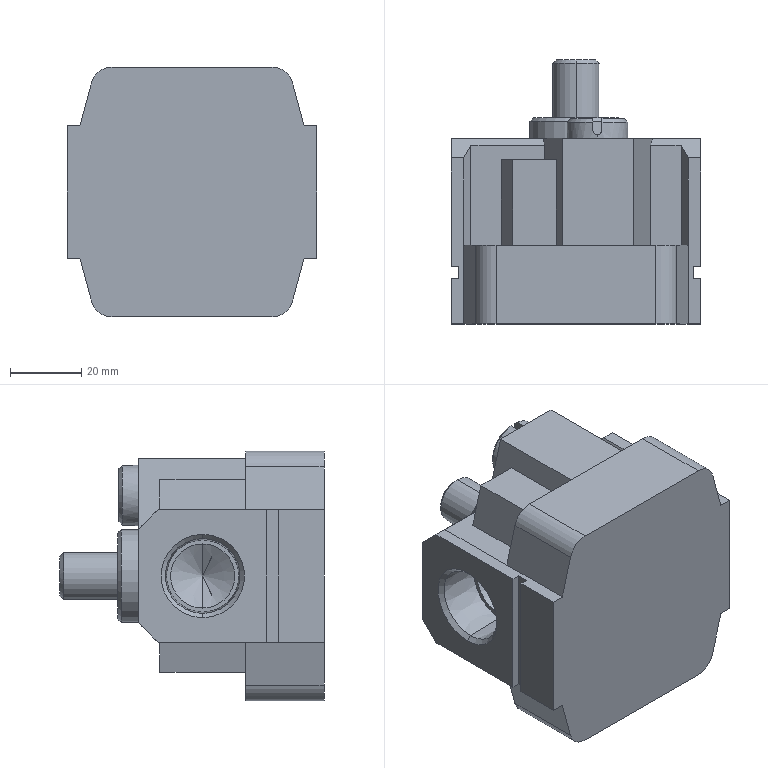Part | STEP file | AC40-04-KSTV-38JNR_AC3009A AL Body-1 | 1 solid | 137 faces | box 70 x 74 x 70 mm | volume 184515 mm3 | plane 71 | cone 34 | cylinder 32 | commonest cylinder face diameters 4.2 x8 5 x8 12 x4 18 x4 2.5 x2 13.2 x2